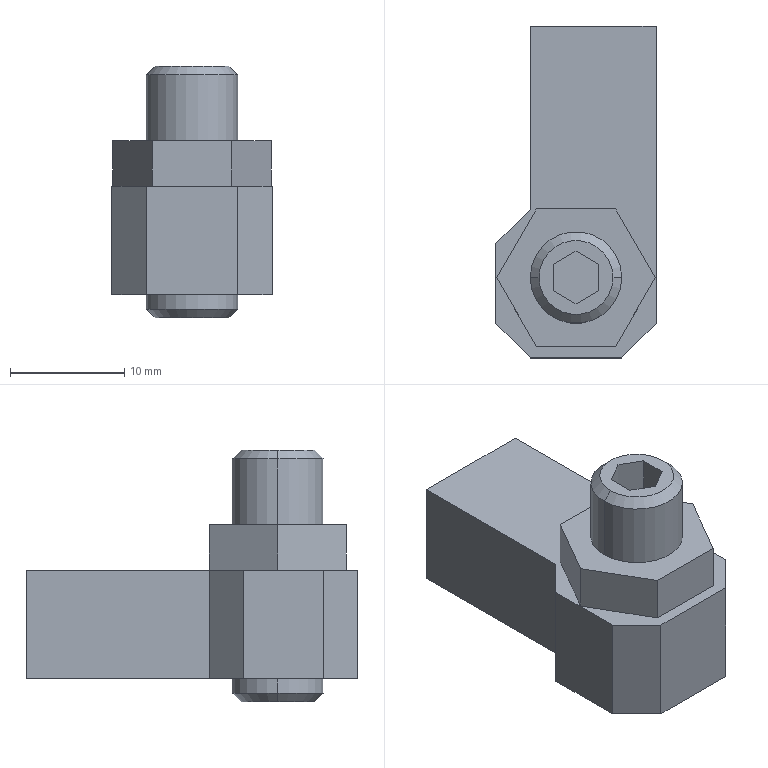Part | SolidWorks | features RefAxis 6, ICE 4, Revolution 3, 3DProfileFeature 2, LPattern 2, Extrusion 1, HoleWzd 1 | 1 solid | 64 faces | box 14 x 29 x 22 mm | volume 4035 mm3 | plane 44 | cylinder 12 | cone 8 | commonest cylinder face diameters 7 x4 7.3 x4 8 x4